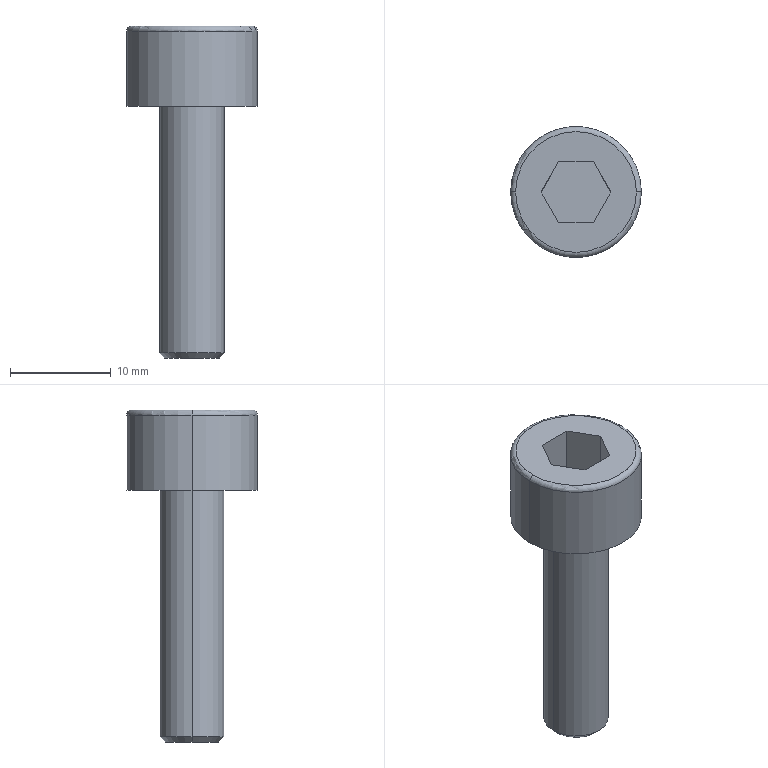Part | CATIA | 1 solid | 18 faces | box 13 x 13 x 33 mm | volume 1675 mm3 | plane 10 | cylinder 4 | torus 2 | cone 2 | commonest cylinder face diameters 6.4 x2 13 x2
STEP:
#1=CARTESIAN_POINT('',(-6.5,0.,0.));
#2=VERTEX_POINT('',#1);
#3=CARTESIAN_POINT('',(6.5,0.,0.));
#4=VERTEX_POINT('',#3);
#5=CARTESIAN_POINT('',(0.,0.,0.));
#6=DIRECTION('',(0.,0.,1.));
#7=AXIS2_PLACEMENT_3D('',#5,#6,$);
#8=CIRCLE('',#7,6.5);
#9=EDGE_CURVE('',#2,#4,#8,.T.);
#10=ORIENTED_EDGE('',*,*,#9,.F.);
#11=CARTESIAN_POINT('',(0.,0.,0.));
#12=DIRECTION('',(0.,0.,1.));
#13=AXIS2_PLACEMENT_3D('',#11,#12,$);
#14=CIRCLE('',#13,6.5);
#15=EDGE_CURVE('',#4,#2,#14,.T.);
#16=ORIENTED_EDGE('',*,*,#15,.F.);
#17=EDGE_LOOP('',(#10,#16));
#18=FACE_OUTER_BOUND('',#17,.T.);
#19=CARTESIAN_POINT('',(-3.2,0.,0.));
#20=VERTEX_POINT('',#19);
#21=CARTESIAN_POINT('',(3.2,0.,0.));
#22=VERTEX_POINT('',#21);
#23=CARTESIAN_POINT('',(0.,0.,0.));
#24=DIRECTION('',(0.,0.,1.));
#25=AXIS2_PLACEMENT_3D('',#23,#24,$);
#26=CIRCLE('',#25,3.2);
#27=EDGE_CURVE('',#20,#22,#26,.F.);
#28=ORIENTED_EDGE('',*,*,#27,.F.);
#29=CARTESIAN_POINT('',(0.,0.,0.));
#30=DIRECTION('',(0.,0.,1.));
#31=AXIS2_PLACEMENT_3D('',#29,#30,$);
#32=CIRCLE('',#31,3.2);
#33=EDGE_CURVE('',#22,#20,#32,.F.);
#34=ORIENTED_EDGE('',*,*,#33,.F.);
#35=EDGE_LOOP('',(#28,#34));
#36=FACE_BOUND('',#35,.T.);
#37=CARTESIAN_POINT('',(0.,0.,0.));
#38=DIRECTION('',(0.,0.,1.));
#39=DIRECTION('',(1.,0.,0.));
#40=AXIS2_PLACEMENT_3D('',#37,#38,#39);
#41=PLANE('',#40);
#42=ADVANCED_FACE('',(#18,#36),#41,.F.);
#43=CARTESIAN_POINT('',(-1.732,-3.,8.));
#44=VERTEX_POINT('',#43);
#45=CARTESIAN_POINT('',(-1.732,-3.,2.));
#46=VERTEX_POINT('',#45);
#47=CARTESIAN_POINT('',(-1.732,-3.,5.));
#48=DIRECTION('',(0.,0.,-1.));
#49=VECTOR('',#48,1.);
#50=LINE('',#47,#49);
#51=EDGE_CURVE('',#44,#46,#50,.T.);
#52=ORIENTED_EDGE('',*,*,#51,.F.);
#53=CARTESIAN_POINT('',(1.732,-3.,8.));
#54=VERTEX_POINT('',#53);
#55=CARTESIAN_POINT('',(0.,-3.,8.));
#56=DIRECTION('',(1.,0.,0.));
#57=VECTOR('',#56,1.);
#58=LINE('',#55,#57);
#59=EDGE_CURVE('',#44,#54,#58,.T.);
#60=ORIENTED_EDGE('',*,*,#59,.T.);
#61=CARTESIAN_POINT('',(1.732,-3.,2.));
#62=VERTEX_POINT('',#61);
#63=CARTESIAN_POINT('',(1.732,-3.,5.));
#64=DIRECTION('',(0.,0.,-1.));
#65=VECTOR('',#64,1.);
#66=LINE('',#63,#65);
#67=EDGE_CURVE('',#54,#62,#66,.T.);
#68=ORIENTED_EDGE('',*,*,#67,.T.);
#69=CARTESIAN_POINT('',(0.,-3.,2.));
#70=DIRECTION('',(1.,0.,0.));
#71=VECTOR('',#70,1.);
#72=LINE('',#69,#71);
#73=EDGE_CURVE('',#46,#62,#72,.T.);
#74=ORIENTED_EDGE('',*,*,#73,.F.);
#75=EDGE_LOOP('',(#52,#60,#68,#74));
#76=FACE_OUTER_BOUND('',#75,.T.);
#77=CARTESIAN_POINT('',(-1.732,-3.,8.));
#78=DIRECTION('',(0.,1.,0.));
#79=DIRECTION('',(1.,0.,0.));
#80=AXIS2_PLACEMENT_3D('',#77,#78,#79);
#81=PLANE('',#80);
#82=ADVANCED_FACE('',(#76),#81,.T.);
#83=CARTESIAN_POINT('',(-3.464,0.,8.));
#84=VERTEX_POINT('',#83);
#85=CARTESIAN_POINT('',(-3.464,0.,2.));
#86=VERTEX_POINT('',#85);
#87=CARTESIAN_POINT('',(-3.464,0.,5.));
#88=DIRECTION('',(0.,0.,-1.));
#89=VECTOR('',#88,1.);
#90=LINE('',#87,#89);
#91=EDGE_CURVE('',#84,#86,#90,.T.);
#92=ORIENTED_EDGE('',*,*,#91,.F.);
#93=CARTESIAN_POINT('',(-2.598,-1.5,8.));
#94=DIRECTION('',(0.5,-0.866,0.));
#95=VECTOR('',#94,1.);
#96=LINE('',#93,#95);
#97=EDGE_CURVE('',#84,#44,#96,.T.);
#98=ORIENTED_EDGE('',*,*,#97,.T.);
#99=ORIENTED_EDGE('',*,*,#51,.T.);
#100=CARTESIAN_POINT('',(-2.598,-1.5,2.));
#101=DIRECTION('',(0.5,-0.866,0.));
#102=VECTOR('',#101,1.);
#103=LINE('',#100,#102);
#104=EDGE_CURVE('',#86,#46,#103,.T.);
#105=ORIENTED_EDGE('',*,*,#104,.F.);
#106=EDGE_LOOP('',(#92,#98,#99,#105));
#107=FACE_OUTER_BOUND('',#106,.T.);
#108=CARTESIAN_POINT('',(-3.464,0.,8.));
#109=DIRECTION('',(0.866,0.5,0.));
#110=DIRECTION('',(0.5,-0.866,0.));
#111=AXIS2_PLACEMENT_3D('',#108,#109,#110);
#112=PLANE('',#111);
#113=ADVANCED_FACE('',(#107),#112,.T.);
#114=ORIENTED_EDGE('',*,*,#67,.F.);
#115=CARTESIAN_POINT('',(3.464,0.,8.));
#116=VERTEX_POINT('',#115);
#117=CARTESIAN_POINT('',(2.598,-1.5,8.));
#118=DIRECTION('',(0.5,0.866,0.));
#119=VECTOR('',#118,1.);
#120=LINE('',#117,#119);
#121=EDGE_CURVE('',#54,#116,#120,.T.);
#122=ORIENTED_EDGE('',*,*,#121,.T.);
#123=CARTESIAN_POINT('',(3.464,0.,2.));
#124=VERTEX_POINT('',#123);
#125=CARTESIAN_POINT('',(3.464,0.,5.));
#126=DIRECTION('',(0.,0.,-1.));
#127=VECTOR('',#126,1.);
#128=LINE('',#125,#127);
#129=EDGE_CURVE('',#116,#124,#128,.T.);
#130=ORIENTED_EDGE('',*,*,#129,.T.);
#131=CARTESIAN_POINT('',(2.598,-1.5,2.));
#132=DIRECTION('',(0.5,0.866,0.));
#133=VECTOR('',#132,1.);
#134=LINE('',#131,#133);
#135=EDGE_CURVE('',#62,#124,#134,.T.);
#136=ORIENTED_EDGE('',*,*,#135,.F.);
#137=EDGE_LOOP('',(#114,#122,#130,#136));
#138=FACE_OUTER_BOUND('',#137,.T.);
#139=CARTESIAN_POINT('',(1.732,-3.,8.));
#140=DIRECTION('',(-0.866,0.5,0.));
#141=DIRECTION('',(0.5,0.866,0.));
#142=AXIS2_PLACEMENT_3D('',#139,#140,#141);
#143=PLANE('',#142);
#144=ADVANCED_FACE('',(#138),#143,.T.);
#145=CARTESIAN_POINT('',(1.732,3.,2.));
#146=VERTEX_POINT('',#145);
#147=CARTESIAN_POINT('',(-1.732,3.,2.));
#148=VERTEX_POINT('',#147);
#149=CARTESIAN_POINT('',(0.,3.,2.));
#150=DIRECTION('',(-1.,0.,0.));
#151=VECTOR('',#150,1.);
#152=LINE('',#149,#151);
#153=EDGE_CURVE('',#146,#148,#152,.T.);
#154=ORIENTED_EDGE('',*,*,#153,.T.);
#155=CARTESIAN_POINT('',(-2.598,1.5,2.));
#156=DIRECTION('',(-0.5,-0.866,0.));
#157=VECTOR('',#156,1.);
#158=LINE('',#155,#157);
#159=EDGE_CURVE('',#148,#86,#158,.T.);
#160=ORIENTED_EDGE('',*,*,#159,.T.);
#161=ORIENTED_EDGE('',*,*,#104,.T.);
#162=ORIENTED_EDGE('',*,*,#73,.T.);
#163=ORIENTED_EDGE('',*,*,#135,.T.);
#164=CARTESIAN_POINT('',(2.598,1.5,2.));
#165=DIRECTION('',(-0.5,0.866,0.));
#166=VECTOR('',#165,1.);
#167=LINE('',#164,#166);
#168=EDGE_CURVE('',#124,#146,#167,.T.);
#169=ORIENTED_EDGE('',*,*,#168,.T.);
#170=EDGE_LOOP('',(#154,#160,#161,#162,#163,#169));
#171=FACE_OUTER_BOUND('',#170,.T.);
#172=CARTESIAN_POINT('',(0.,0.,2.));
#173=DIRECTION('',(0.,0.,1.));
#174=DIRECTION('',(1.,0.,0.));
#175=AXIS2_PLACEMENT_3D('',#172,#173,#174);
#176=PLANE('',#175);
#177=ADVANCED_FACE('',(#171),#176,.T.);
#178=CARTESIAN_POINT('',(-1.732,3.,8.));
#179=VERTEX_POINT('',#178);
#180=CARTESIAN_POINT('',(-1.732,3.,5.));
#181=DIRECTION('',(0.,0.,-1.));
#182=VECTOR('',#181,1.);
#183=LINE('',#180,#182);
#184=EDGE_CURVE('',#179,#148,#183,.T.);
#185=ORIENTED_EDGE('',*,*,#184,.F.);
#186=CARTESIAN_POINT('',(-2.598,1.5,8.));
#187=DIRECTION('',(-0.5,-0.866,0.));
#188=VECTOR('',#187,1.);
#189=LINE('',#186,#188);
#190=EDGE_CURVE('',#179,#84,#189,.T.);
#191=ORIENTED_EDGE('',*,*,#190,.T.);
#192=ORIENTED_EDGE('',*,*,#91,.T.);
#193=ORIENTED_EDGE('',*,*,#159,.F.);
#194=EDGE_LOOP('',(#185,#191,#192,#193));
#195=FACE_OUTER_BOUND('',#194,.T.);
#196=CARTESIAN_POINT('',(-1.732,3.,8.));
#197=DIRECTION('',(0.866,-0.5,0.));
#198=DIRECTION('',(-0.5,-0.866,0.));
#199=AXIS2_PLACEMENT_3D('',#196,#197,#198);
#200=PLANE('',#199);
#201=ADVANCED_FACE('',(#195),#200,.T.);
#202=ORIENTED_EDGE('',*,*,#129,.F.);
#203=CARTESIAN_POINT('',(1.732,3.,8.));
#204=VERTEX_POINT('',#203);
#205=CARTESIAN_POINT('',(2.598,1.5,8.));
#206=DIRECTION('',(-0.5,0.866,0.));
#207=VECTOR('',#206,1.);
#208=LINE('',#205,#207);
#209=EDGE_CURVE('',#116,#204,#208,.T.);
#210=ORIENTED_EDGE('',*,*,#209,.T.);
#211=CARTESIAN_POINT('',(1.732,3.,5.));
#212=DIRECTION('',(0.,0.,-1.));
#213=VECTOR('',#212,1.);
#214=LINE('',#211,#213);
#215=EDGE_CURVE('',#204,#146,#214,.T.);
#216=ORIENTED_EDGE('',*,*,#215,.T.);
#217=ORIENTED_EDGE('',*,*,#168,.F.);
#218=EDGE_LOOP('',(#202,#210,#216,#217));
#219=FACE_OUTER_BOUND('',#218,.T.);
#220=CARTESIAN_POINT('',(3.464,0.,8.));
#221=DIRECTION('',(-0.866,-0.5,0.));
#222=DIRECTION('',(-0.5,0.866,0.));
#223=AXIS2_PLACEMENT_3D('',#220,#221,#222);
#224=PLANE('',#223);
#225=ADVANCED_FACE('',(#219),#224,.T.);
#226=ORIENTED_EDGE('',*,*,#215,.F.);
#227=CARTESIAN_POINT('',(0.,3.,8.));
#228=DIRECTION('',(-1.,0.,0.));
#229=VECTOR('',#228,1.);
#230=LINE('',#227,#229);
#231=EDGE_CURVE('',#204,#179,#230,.T.);
#232=ORIENTED_EDGE('',*,*,#231,.T.);
#233=ORIENTED_EDGE('',*,*,#184,.T.);
#234=ORIENTED_EDGE('',*,*,#153,.F.);
#235=EDGE_LOOP('',(#226,#232,#233,#234));
#236=FACE_OUTER_BOUND('',#235,.T.);
#237=CARTESIAN_POINT('',(1.732,3.,8.));
#238=DIRECTION('',(0.,-1.,0.));
#239=DIRECTION('',(-1.,0.,0.));
#240=AXIS2_PLACEMENT_3D('',#237,#238,#239);
#241=PLANE('',#240);
#242=ADVANCED_FACE('',(#236),#241,.T.);
#243=CARTESIAN_POINT('',(-6.,0.000000322,8.));
#244=VERTEX_POINT('',#243);
#245=CARTESIAN_POINT('',(6.,0.,8.));
#246=VERTEX_POINT('',#245);
#247=CARTESIAN_POINT('',(0.,0.,8.));
#248=DIRECTION('',(0.,0.,1.));
#249=AXIS2_PLACEMENT_3D('',#247,#248,$);
#250=CIRCLE('',#249,6.);
#251=EDGE_CURVE('',#244,#246,#250,.T.);
#252=ORIENTED_EDGE('',*,*,#251,.T.);
#253=CARTESIAN_POINT('',(0.,0.,8.));
#254=DIRECTION('',(0.,0.,1.));
#255=AXIS2_PLACEMENT_3D('',#253,#254,$);
#256=CIRCLE('',#255,6.);
#257=EDGE_CURVE('',#246,#244,#256,.T.);
#258=ORIENTED_EDGE('',*,*,#257,.T.);
#259=EDGE_LOOP('',(#252,#258));
#260=FACE_OUTER_BOUND('',#259,.T.);
#261=ORIENTED_EDGE('',*,*,#121,.F.);
#262=ORIENTED_EDGE('',*,*,#59,.F.);
#263=ORIENTED_EDGE('',*,*,#97,.F.);
#264=ORIENTED_EDGE('',*,*,#190,.F.);
#265=ORIENTED_EDGE('',*,*,#231,.F.);
#266=ORIENTED_EDGE('',*,*,#209,.F.);
#267=EDGE_LOOP('',(#261,#262,#263,#264,#265,#266));
#268=FACE_BOUND('',#267,.T.);
#269=CARTESIAN_POINT('',(0.,0.,8.));
#270=DIRECTION('',(0.,0.,1.));
#271=DIRECTION('',(1.,0.,0.));
#272=AXIS2_PLACEMENT_3D('',#269,#270,#271);
#273=PLANE('',#272);
#274=ADVANCED_FACE('',(#260,#268),#273,.T.);
#275=CARTESIAN_POINT('',(-6.5,0.,7.5));
#276=VERTEX_POINT('',#275);
#277=CARTESIAN_POINT('',(-6.5,0.,4.));
#278=DIRECTION('',(0.,0.,1.));
#279=VECTOR('',#278,1.);
#280=LINE('',#277,#279);
#281=EDGE_CURVE('',#2,#276,#280,.T.);
#282=ORIENTED_EDGE('',*,*,#281,.F.);
#283=ORIENTED_EDGE('',*,*,#9,.T.);
#284=CARTESIAN_POINT('',(6.5,0.,7.5));
#285=VERTEX_POINT('',#284);
#286=CARTESIAN_POINT('',(6.5,0.,4.));
#287=DIRECTION('',(0.,0.,1.));
#288=VECTOR('',#287,1.);
#289=LINE('',#286,#288);
#290=EDGE_CURVE('',#4,#285,#289,.T.);
#291=ORIENTED_EDGE('',*,*,#290,.T.);
#292=CARTESIAN_POINT('',(0.,0.,7.5));
#293=DIRECTION('',(0.,0.,1.));
#294=AXIS2_PLACEMENT_3D('',#292,#293,$);
#295=CIRCLE('',#294,6.5);
#296=EDGE_CURVE('',#276,#285,#295,.T.);
#297=ORIENTED_EDGE('',*,*,#296,.F.);
#298=EDGE_LOOP('',(#282,#283,#291,#297));
#299=FACE_OUTER_BOUND('',#298,.T.);
#300=CARTESIAN_POINT('',(0.,0.,4.));
#301=DIRECTION('',(0.,0.,1.));
#302=DIRECTION('',(1.,0.,0.));
#303=AXIS2_PLACEMENT_3D('',#300,#301,#302);
#304=CYLINDRICAL_SURFACE('',#303,6.5);
#305=ADVANCED_FACE('',(#299),#304,.T.);
#306=ORIENTED_EDGE('',*,*,#290,.F.);
#307=ORIENTED_EDGE('',*,*,#15,.T.);
#308=ORIENTED_EDGE('',*,*,#281,.T.);
#309=CARTESIAN_POINT('',(0.,0.,7.5));
#310=DIRECTION('',(0.,0.,1.));
#311=AXIS2_PLACEMENT_3D('',#309,#310,$);
#312=CIRCLE('',#311,6.5);
#313=EDGE_CURVE('',#285,#276,#312,.T.);
#314=ORIENTED_EDGE('',*,*,#313,.F.);
#315=EDGE_LOOP('',(#306,#307,#308,#314));
#316=FACE_OUTER_BOUND('',#315,.T.);
#317=ADVANCED_FACE('',(#316),#304,.T.);
#318=CARTESIAN_POINT('',(-6.,0.,7.5));
#319=DIRECTION('',(0.,1.,0.));
#320=AXIS2_PLACEMENT_3D('',#318,#319,$);
#321=CIRCLE('',#320,0.5);
#322=EDGE_CURVE('',#244,#276,#321,.F.);
#323=ORIENTED_EDGE('',*,*,#322,.T.);
#324=ORIENTED_EDGE('',*,*,#296,.T.);
#325=CARTESIAN_POINT('',(6.,0.,7.5));
#326=DIRECTION('',(0.,-1.,0.));
#327=AXIS2_PLACEMENT_3D('',#325,#326,$);
#328=CIRCLE('',#327,0.5);
#329=EDGE_CURVE('',#246,#285,#328,.F.);
#330=ORIENTED_EDGE('',*,*,#329,.F.);
#331=ORIENTED_EDGE('',*,*,#251,.F.);
#332=EDGE_LOOP('',(#323,#324,#330,#331));
#333=FACE_OUTER_BOUND('',#332,.T.);
#334=CARTESIAN_POINT('',(0.,0.,7.5));
#335=DIRECTION('',(0.,0.,1.));
#336=DIRECTION('',(-0.9461,0.3239,0.));
#337=AXIS2_PLACEMENT_3D('',#334,#335,#336);
#338=TOROIDAL_SURFACE('',#337,6.,0.5);
#339=ADVANCED_FACE('',(#333),#338,.T.);
#340=ORIENTED_EDGE('',*,*,#329,.T.);
#341=ORIENTED_EDGE('',*,*,#313,.T.);
#342=ORIENTED_EDGE('',*,*,#322,.F.);
#343=ORIENTED_EDGE('',*,*,#257,.F.);
#344=EDGE_LOOP('',(#340,#341,#342,#343));
#345=FACE_OUTER_BOUND('',#344,.T.);
#346=CARTESIAN_POINT('',(0.,0.,7.5));
#347=DIRECTION('',(0.,0.,1.));
#348=DIRECTION('',(1.,0.,0.));
#349=AXIS2_PLACEMENT_3D('',#346,#347,#348);
#350=TOROIDAL_SURFACE('',#349,6.,0.5);
#351=ADVANCED_FACE('',(#345),#350,.T.);
#352=CARTESIAN_POINT('',(3.2,0.,-24.5));
#353=VERTEX_POINT('',#352);
#354=CARTESIAN_POINT('',(3.2,0.,-12.5));
#355=DIRECTION('',(0.,0.,-1.));
#356=VECTOR('',#355,1.);
#357=LINE('',#354,#356);
#358=EDGE_CURVE('',#22,#353,#357,.T.);
#359=ORIENTED_EDGE('',*,*,#358,.F.);
#360=ORIENTED_EDGE('',*,*,#33,.T.);
#361=CARTESIAN_POINT('',(-3.2,0.,-24.5));
#362=VERTEX_POINT('',#361);
#363=CARTESIAN_POINT('',(-3.2,0.,-12.5));
#364=DIRECTION('',(0.,0.,-1.));
#365=VECTOR('',#364,1.);
#366=LINE('',#363,#365);
#367=EDGE_CURVE('',#20,#362,#366,.T.);
#368=ORIENTED_EDGE('',*,*,#367,.T.);
#369=CARTESIAN_POINT('',(0.,0.,-24.5));
#370=DIRECTION('',(0.,0.,-1.));
#371=AXIS2_PLACEMENT_3D('',#369,#370,$);
#372=CIRCLE('',#371,3.2);
#373=EDGE_CURVE('',#353,#362,#372,.T.);
#374=ORIENTED_EDGE('',*,*,#373,.F.);
#375=EDGE_LOOP('',(#359,#360,#368,#374));
#376=FACE_OUTER_BOUND('',#375,.T.);
#377=CARTESIAN_POINT('',(0.,0.,-12.5));
#378=DIRECTION('',(0.,0.,-1.));
#379=DIRECTION('',(1.,0.,0.));
#380=AXIS2_PLACEMENT_3D('',#377,#378,#379);
#381=CYLINDRICAL_SURFACE('',#380,3.2);
#382=ADVANCED_FACE('',(#376),#381,.T.);
#383=ORIENTED_EDGE('',*,*,#367,.F.);
#384=ORIENTED_EDGE('',*,*,#27,.T.);
#385=ORIENTED_EDGE('',*,*,#358,.T.);
#386=CARTESIAN_POINT('',(0.,0.,-24.5));
#387=DIRECTION('',(0.,0.,-1.));
#388=AXIS2_PLACEMENT_3D('',#386,#387,$);
#389=CIRCLE('',#388,3.2);
#390=EDGE_CURVE('',#362,#353,#389,.T.);
#391=ORIENTED_EDGE('',*,*,#390,.F.);
#392=EDGE_LOOP('',(#383,#384,#385,#391));
#393=FACE_OUTER_BOUND('',#392,.T.);
#394=ADVANCED_FACE('',(#393),#381,.T.);
#395=CARTESIAN_POINT('',(-2.7,-0.000000824,-25.));
#396=VERTEX_POINT('',#395);
#397=CARTESIAN_POINT('',(2.7,0.,-25.));
#398=VERTEX_POINT('',#397);
#399=CARTESIAN_POINT('',(0.,0.,-25.));
#400=DIRECTION('',(0.,0.,-1.));
#401=AXIS2_PLACEMENT_3D('',#399,#400,$);
#402=CIRCLE('',#401,2.7);
#403=EDGE_CURVE('',#396,#398,#402,.T.);
#404=ORIENTED_EDGE('',*,*,#403,.T.);
#405=CARTESIAN_POINT('',(0.,0.,-25.));
#406=DIRECTION('',(0.,0.,-1.));
#407=AXIS2_PLACEMENT_3D('',#405,#406,$);
#408=CIRCLE('',#407,2.7);
#409=EDGE_CURVE('',#398,#396,#408,.T.);
#410=ORIENTED_EDGE('',*,*,#409,.T.);
#411=EDGE_LOOP('',(#404,#410));
#412=FACE_OUTER_BOUND('',#411,.T.);
#413=CARTESIAN_POINT('',(0.,0.,-25.));
#414=DIRECTION('',(0.,0.,-1.));
#415=DIRECTION('',(1.,0.,0.));
#416=AXIS2_PLACEMENT_3D('',#413,#414,#415);
#417=PLANE('',#416);
#418=ADVANCED_FACE('',(#412),#417,.T.);
#419=CARTESIAN_POINT('',(-2.95,0.,-24.75));
#420=DIRECTION('',(-0.7071,0.,0.7071));
#421=VECTOR('',#420,1.);
#422=LINE('',#419,#421);
#423=EDGE_CURVE('',#396,#362,#422,.T.);
#424=ORIENTED_EDGE('',*,*,#423,.T.);
#425=ORIENTED_EDGE('',*,*,#390,.T.);
#426=CARTESIAN_POINT('',(2.95,0.,-24.75));
#427=DIRECTION('',(0.7071,0.,0.7071));
#428=VECTOR('',#427,1.);
#429=LINE('',#426,#428);
#430=EDGE_CURVE('',#398,#353,#429,.T.);
#431=ORIENTED_EDGE('',*,*,#430,.F.);
#432=ORIENTED_EDGE('',*,*,#403,.F.);
#433=EDGE_LOOP('',(#424,#425,#431,#432));
#434=FACE_OUTER_BOUND('',#433,.T.);
#435=CARTESIAN_POINT('',(0.,0.,-27.7));
#436=DIRECTION('',(0.,0.,1.));
#437=DIRECTION('',(-0.9723,-0.2337,0.));
#438=AXIS2_PLACEMENT_3D('',#435,#436,#437);
#439=CONICAL_SURFACE('',#438,0.,0.7854);
#440=ADVANCED_FACE('',(#434),#439,.T.);
#441=ORIENTED_EDGE('',*,*,#430,.T.);
#442=ORIENTED_EDGE('',*,*,#373,.T.);
#443=ORIENTED_EDGE('',*,*,#423,.F.);
#444=ORIENTED_EDGE('',*,*,#409,.F.);
#445=EDGE_LOOP('',(#441,#442,#443,#444));
#446=FACE_OUTER_BOUND('',#445,.T.);
#447=CARTESIAN_POINT('',(0.,0.,-27.7));
#448=DIRECTION('',(0.,0.,1.));
#449=DIRECTION('',(1.,0.,0.));
#450=AXIS2_PLACEMENT_3D('',#447,#448,#449);
#451=CONICAL_SURFACE('',#450,0.,0.7854);
#452=ADVANCED_FACE('',(#446),#451,.T.);
#453=CLOSED_SHELL('',(#42,#82,#113,#144,#177,#201,#225,#242,#274,#305,#317,#339,#351,#382,#394,#418,#440,#452));
#454=MANIFOLD_SOLID_BREP('',#453);
#455=(LENGTH_UNIT()NAMED_UNIT(*)SI_UNIT(.MILLI.,.METRE.));
#456=UNCERTAINTY_MEASURE_WITH_UNIT(LENGTH_MEASURE(0.005),#455,'','');
#457=(NAMED_UNIT(*)PLANE_ANGLE_UNIT()SI_UNIT($,.RADIAN.));
#458=(NAMED_UNIT(*)SI_UNIT($,.STERADIAN.)SOLID_ANGLE_UNIT());
#459=(GEOMETRIC_REPRESENTATION_CONTEXT(3)GLOBAL_UNCERTAINTY_ASSIGNED_CONTEXT((#456))GLOBAL_UNIT_ASSIGNED_CONTEXT((#455,#457,#458))REPRESENTATION_CONTEXT('',''));
#460=ADVANCED_BREP_SHAPE_REPRESENTATION('',(#454),#459);